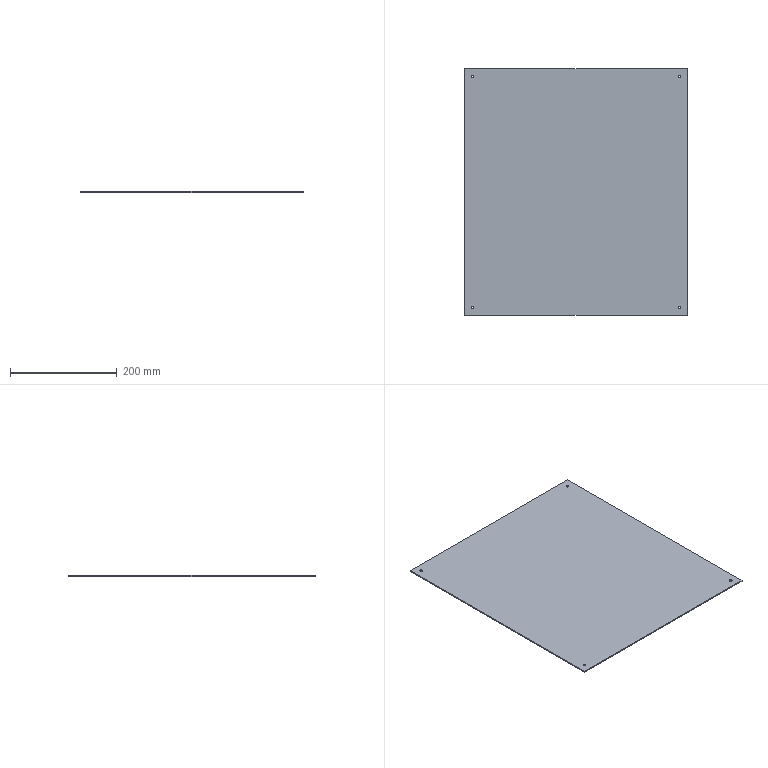Part | STEP file | PN_0004 (cover plate) | 1 solid | 14 faces | box 418 x 463 x 2 mm | volume 386911 mm3 | cylinder 8 | plane 6 | commonest cylinder face diameters 5 x8
STEP:
#1=CARTESIAN_POINT('',(0.,0.,0.));
#2=DIRECTION('',(0.,0.,1.));
#3=DIRECTION('',(1.,0.,0.));
#4=AXIS2_PLACEMENT_3D('',#1,#2,#3);
#5=CARTESIAN_POINT('',(-191.5,216.5,-2.));
#6=VERTEX_POINT('',#5);
#7=CARTESIAN_POINT('',(-191.5,216.5,0.));
#8=VERTEX_POINT('',#7);
#9=CARTESIAN_POINT('',(-191.5,216.5,0.));
#10=DIRECTION('',(0.,0.,1.));
#11=VECTOR('',#10,1.);
#12=LINE('',#9,#11);
#13=CARTESIAN_POINT('',(-194.,216.5,0.));
#14=DIRECTION('',(0.,0.,1.));
#15=DIRECTION('',(1.,0.,0.));
#16=AXIS2_PLACEMENT_3D('',#13,#14,#15);
#17=CYLINDRICAL_SURFACE('',#16,2.5);
#18=CARTESIAN_POINT('',(6.283,0.));
#19=DIRECTION('',(0.,1.));
#20=VECTOR('',#19,1.);
#21=LINE('',#18,#20);
#22=(GEOMETRIC_REPRESENTATION_CONTEXT(2)PARAMETRIC_REPRESENTATION_CONTEXT()REPRESENTATION_CONTEXT('',''));
#23=DEFINITIONAL_REPRESENTATION('',(#21),#22);
#24=PCURVE('',#17,#23);
#25=CARTESIAN_POINT('',(-194.,216.5,0.));
#26=DIRECTION('',(0.,0.,1.));
#27=DIRECTION('',(1.,0.,0.));
#28=AXIS2_PLACEMENT_3D('',#25,#26,#27);
#29=CYLINDRICAL_SURFACE('',#28,2.5);
#30=CARTESIAN_POINT('',(0.,0.));
#31=DIRECTION('',(0.,1.));
#32=VECTOR('',#31,1.);
#33=LINE('',#30,#32);
#34=(GEOMETRIC_REPRESENTATION_CONTEXT(2)PARAMETRIC_REPRESENTATION_CONTEXT()REPRESENTATION_CONTEXT('',''));
#35=DEFINITIONAL_REPRESENTATION('',(#33),#34);
#36=PCURVE('',#29,#35);
#37=SURFACE_CURVE('',#12,(#24,#36),.PCURVE_S1.);
#38=EDGE_CURVE('',#6,#8,#37,.T.);
#39=ORIENTED_EDGE('',*,*,#38,.T.);
#40=CARTESIAN_POINT('',(-196.5,216.5,0.));
#41=VERTEX_POINT('',#40);
#42=CARTESIAN_POINT('',(-194.,216.5,0.));
#43=DIRECTION('',(0.,0.,1.));
#44=DIRECTION('',(1.,0.,0.));
#45=AXIS2_PLACEMENT_3D('',#42,#43,#44);
#46=CIRCLE('',#45,2.5);
#47=CARTESIAN_POINT('',(0.,0.));
#48=DIRECTION('',(1.,0.));
#49=VECTOR('',#48,1.);
#50=LINE('',#47,#49);
#51=(GEOMETRIC_REPRESENTATION_CONTEXT(2)PARAMETRIC_REPRESENTATION_CONTEXT()REPRESENTATION_CONTEXT('',''));
#52=DEFINITIONAL_REPRESENTATION('',(#50),#51);
#53=PCURVE('',#17,#52);
#54=CARTESIAN_POINT('',(0.,0.,0.));
#55=DIRECTION('',(0.,0.,1.));
#56=DIRECTION('',(1.,0.,0.));
#57=AXIS2_PLACEMENT_3D('',#54,#55,#56);
#58=PLANE('',#57);
#59=CARTESIAN_POINT('',(-194.,216.5));
#60=DIRECTION('',(1.,0.));
#61=AXIS2_PLACEMENT_2D('',#59,#60);
#62=CIRCLE('',#61,2.5);
#63=(GEOMETRIC_REPRESENTATION_CONTEXT(2)PARAMETRIC_REPRESENTATION_CONTEXT()REPRESENTATION_CONTEXT('',''));
#64=DEFINITIONAL_REPRESENTATION('',(#62),#63);
#65=PCURVE('',#58,#64);
#66=SURFACE_CURVE('',#46,(#53,#65),.PCURVE_S1.);
#67=EDGE_CURVE('',#41,#8,#66,.T.);
#68=ORIENTED_EDGE('',*,*,#67,.F.);
#69=CARTESIAN_POINT('',(-196.5,216.5,-2.));
#70=VERTEX_POINT('',#69);
#71=CARTESIAN_POINT('',(-196.5,216.5,0.));
#72=DIRECTION('',(0.,0.,1.));
#73=VECTOR('',#72,1.);
#74=LINE('',#71,#73);
#75=CARTESIAN_POINT('',(3.142,0.));
#76=DIRECTION('',(0.,1.));
#77=VECTOR('',#76,1.);
#78=LINE('',#75,#77);
#79=(GEOMETRIC_REPRESENTATION_CONTEXT(2)PARAMETRIC_REPRESENTATION_CONTEXT()REPRESENTATION_CONTEXT('',''));
#80=DEFINITIONAL_REPRESENTATION('',(#78),#79);
#81=PCURVE('',#17,#80);
#82=CARTESIAN_POINT('',(3.142,0.));
#83=DIRECTION('',(0.,1.));
#84=VECTOR('',#83,1.);
#85=LINE('',#82,#84);
#86=(GEOMETRIC_REPRESENTATION_CONTEXT(2)PARAMETRIC_REPRESENTATION_CONTEXT()REPRESENTATION_CONTEXT('',''));
#87=DEFINITIONAL_REPRESENTATION('',(#85),#86);
#88=PCURVE('',#29,#87);
#89=SURFACE_CURVE('',#74,(#81,#88),.PCURVE_S1.);
#90=EDGE_CURVE('',#70,#41,#89,.T.);
#91=ORIENTED_EDGE('',*,*,#90,.F.);
#92=CARTESIAN_POINT('',(-194.,216.5,-2.));
#93=DIRECTION('',(0.,0.,1.));
#94=DIRECTION('',(1.,0.,0.));
#95=AXIS2_PLACEMENT_3D('',#92,#93,#94);
#96=CIRCLE('',#95,2.5);
#97=CARTESIAN_POINT('',(0.,-2.));
#98=DIRECTION('',(1.,0.));
#99=VECTOR('',#98,1.);
#100=LINE('',#97,#99);
#101=(GEOMETRIC_REPRESENTATION_CONTEXT(2)PARAMETRIC_REPRESENTATION_CONTEXT()REPRESENTATION_CONTEXT('',''));
#102=DEFINITIONAL_REPRESENTATION('',(#100),#101);
#103=PCURVE('',#17,#102);
#104=CARTESIAN_POINT('',(0.,0.,-2.));
#105=DIRECTION('',(0.,0.,1.));
#106=DIRECTION('',(1.,0.,0.));
#107=AXIS2_PLACEMENT_3D('',#104,#105,#106);
#108=PLANE('',#107);
#109=CARTESIAN_POINT('',(-194.,216.5));
#110=DIRECTION('',(1.,0.));
#111=AXIS2_PLACEMENT_2D('',#109,#110);
#112=CIRCLE('',#111,2.5);
#113=(GEOMETRIC_REPRESENTATION_CONTEXT(2)PARAMETRIC_REPRESENTATION_CONTEXT()REPRESENTATION_CONTEXT('',''));
#114=DEFINITIONAL_REPRESENTATION('',(#112),#113);
#115=PCURVE('',#108,#114);
#116=SURFACE_CURVE('',#96,(#103,#115),.PCURVE_S1.);
#117=EDGE_CURVE('',#70,#6,#116,.T.);
#118=ORIENTED_EDGE('',*,*,#117,.T.);
#119=EDGE_LOOP('',(#39,#68,#91,#118));
#120=FACE_BOUND('',#119,.F.);
#121=ADVANCED_FACE('',(#120),#17,.F.);
#122=CARTESIAN_POINT('',(-191.5,-216.5,-2.));
#123=VERTEX_POINT('',#122);
#124=CARTESIAN_POINT('',(-191.5,-216.5,0.));
#125=VERTEX_POINT('',#124);
#126=CARTESIAN_POINT('',(-191.5,-216.5,0.));
#127=DIRECTION('',(0.,0.,1.));
#128=VECTOR('',#127,1.);
#129=LINE('',#126,#128);
#130=CARTESIAN_POINT('',(-194.,-216.5,0.));
#131=DIRECTION('',(0.,0.,1.));
#132=DIRECTION('',(1.,0.,0.));
#133=AXIS2_PLACEMENT_3D('',#130,#131,#132);
#134=CYLINDRICAL_SURFACE('',#133,2.5);
#135=CARTESIAN_POINT('',(6.283,0.));
#136=DIRECTION('',(0.,1.));
#137=VECTOR('',#136,1.);
#138=LINE('',#135,#137);
#139=(GEOMETRIC_REPRESENTATION_CONTEXT(2)PARAMETRIC_REPRESENTATION_CONTEXT()REPRESENTATION_CONTEXT('',''));
#140=DEFINITIONAL_REPRESENTATION('',(#138),#139);
#141=PCURVE('',#134,#140);
#142=CARTESIAN_POINT('',(-194.,-216.5,0.));
#143=DIRECTION('',(0.,0.,1.));
#144=DIRECTION('',(1.,0.,0.));
#145=AXIS2_PLACEMENT_3D('',#142,#143,#144);
#146=CYLINDRICAL_SURFACE('',#145,2.5);
#147=CARTESIAN_POINT('',(0.,0.));
#148=DIRECTION('',(0.,1.));
#149=VECTOR('',#148,1.);
#150=LINE('',#147,#149);
#151=(GEOMETRIC_REPRESENTATION_CONTEXT(2)PARAMETRIC_REPRESENTATION_CONTEXT()REPRESENTATION_CONTEXT('',''));
#152=DEFINITIONAL_REPRESENTATION('',(#150),#151);
#153=PCURVE('',#146,#152);
#154=SURFACE_CURVE('',#129,(#141,#153),.PCURVE_S1.);
#155=EDGE_CURVE('',#123,#125,#154,.T.);
#156=ORIENTED_EDGE('',*,*,#155,.T.);
#157=CARTESIAN_POINT('',(-196.5,-216.5,0.));
#158=VERTEX_POINT('',#157);
#159=CARTESIAN_POINT('',(-194.,-216.5,0.));
#160=DIRECTION('',(0.,0.,1.));
#161=DIRECTION('',(1.,0.,0.));
#162=AXIS2_PLACEMENT_3D('',#159,#160,#161);
#163=CIRCLE('',#162,2.5);
#164=CARTESIAN_POINT('',(0.,0.));
#165=DIRECTION('',(1.,0.));
#166=VECTOR('',#165,1.);
#167=LINE('',#164,#166);
#168=(GEOMETRIC_REPRESENTATION_CONTEXT(2)PARAMETRIC_REPRESENTATION_CONTEXT()REPRESENTATION_CONTEXT('',''));
#169=DEFINITIONAL_REPRESENTATION('',(#167),#168);
#170=PCURVE('',#134,#169);
#171=CARTESIAN_POINT('',(-194.,-216.5));
#172=DIRECTION('',(1.,0.));
#173=AXIS2_PLACEMENT_2D('',#171,#172);
#174=CIRCLE('',#173,2.5);
#175=(GEOMETRIC_REPRESENTATION_CONTEXT(2)PARAMETRIC_REPRESENTATION_CONTEXT()REPRESENTATION_CONTEXT('',''));
#176=DEFINITIONAL_REPRESENTATION('',(#174),#175);
#177=PCURVE('',#58,#176);
#178=SURFACE_CURVE('',#163,(#170,#177),.PCURVE_S1.);
#179=EDGE_CURVE('',#158,#125,#178,.T.);
#180=ORIENTED_EDGE('',*,*,#179,.F.);
#181=CARTESIAN_POINT('',(-196.5,-216.5,-2.));
#182=VERTEX_POINT('',#181);
#183=CARTESIAN_POINT('',(-196.5,-216.5,0.));
#184=DIRECTION('',(0.,0.,1.));
#185=VECTOR('',#184,1.);
#186=LINE('',#183,#185);
#187=CARTESIAN_POINT('',(3.142,0.));
#188=DIRECTION('',(0.,1.));
#189=VECTOR('',#188,1.);
#190=LINE('',#187,#189);
#191=(GEOMETRIC_REPRESENTATION_CONTEXT(2)PARAMETRIC_REPRESENTATION_CONTEXT()REPRESENTATION_CONTEXT('',''));
#192=DEFINITIONAL_REPRESENTATION('',(#190),#191);
#193=PCURVE('',#134,#192);
#194=CARTESIAN_POINT('',(3.142,0.));
#195=DIRECTION('',(0.,1.));
#196=VECTOR('',#195,1.);
#197=LINE('',#194,#196);
#198=(GEOMETRIC_REPRESENTATION_CONTEXT(2)PARAMETRIC_REPRESENTATION_CONTEXT()REPRESENTATION_CONTEXT('',''));
#199=DEFINITIONAL_REPRESENTATION('',(#197),#198);
#200=PCURVE('',#146,#199);
#201=SURFACE_CURVE('',#186,(#193,#200),.PCURVE_S1.);
#202=EDGE_CURVE('',#182,#158,#201,.T.);
#203=ORIENTED_EDGE('',*,*,#202,.F.);
#204=CARTESIAN_POINT('',(-194.,-216.5,-2.));
#205=DIRECTION('',(0.,0.,1.));
#206=DIRECTION('',(1.,0.,0.));
#207=AXIS2_PLACEMENT_3D('',#204,#205,#206);
#208=CIRCLE('',#207,2.5);
#209=CARTESIAN_POINT('',(0.,-2.));
#210=DIRECTION('',(1.,0.));
#211=VECTOR('',#210,1.);
#212=LINE('',#209,#211);
#213=(GEOMETRIC_REPRESENTATION_CONTEXT(2)PARAMETRIC_REPRESENTATION_CONTEXT()REPRESENTATION_CONTEXT('',''));
#214=DEFINITIONAL_REPRESENTATION('',(#212),#213);
#215=PCURVE('',#134,#214);
#216=CARTESIAN_POINT('',(-194.,-216.5));
#217=DIRECTION('',(1.,0.));
#218=AXIS2_PLACEMENT_2D('',#216,#217);
#219=CIRCLE('',#218,2.5);
#220=(GEOMETRIC_REPRESENTATION_CONTEXT(2)PARAMETRIC_REPRESENTATION_CONTEXT()REPRESENTATION_CONTEXT('',''));
#221=DEFINITIONAL_REPRESENTATION('',(#219),#220);
#222=PCURVE('',#108,#221);
#223=SURFACE_CURVE('',#208,(#215,#222),.PCURVE_S1.);
#224=EDGE_CURVE('',#182,#123,#223,.T.);
#225=ORIENTED_EDGE('',*,*,#224,.T.);
#226=EDGE_LOOP('',(#156,#180,#203,#225));
#227=FACE_BOUND('',#226,.F.);
#228=ADVANCED_FACE('',(#227),#134,.F.);
#229=CARTESIAN_POINT('',(196.5,-216.5,-2.));
#230=VERTEX_POINT('',#229);
#231=CARTESIAN_POINT('',(196.5,-216.5,0.));
#232=VERTEX_POINT('',#231);
#233=CARTESIAN_POINT('',(196.5,-216.5,0.));
#234=DIRECTION('',(0.,0.,1.));
#235=VECTOR('',#234,1.);
#236=LINE('',#233,#235);
#237=CARTESIAN_POINT('',(194.,-216.5,0.));
#238=DIRECTION('',(0.,0.,1.));
#239=DIRECTION('',(1.,0.,0.));
#240=AXIS2_PLACEMENT_3D('',#237,#238,#239);
#241=CYLINDRICAL_SURFACE('',#240,2.5);
#242=CARTESIAN_POINT('',(6.283,0.));
#243=DIRECTION('',(0.,1.));
#244=VECTOR('',#243,1.);
#245=LINE('',#242,#244);
#246=(GEOMETRIC_REPRESENTATION_CONTEXT(2)PARAMETRIC_REPRESENTATION_CONTEXT()REPRESENTATION_CONTEXT('',''));
#247=DEFINITIONAL_REPRESENTATION('',(#245),#246);
#248=PCURVE('',#241,#247);
#249=CARTESIAN_POINT('',(194.,-216.5,0.));
#250=DIRECTION('',(0.,0.,1.));
#251=DIRECTION('',(1.,0.,0.));
#252=AXIS2_PLACEMENT_3D('',#249,#250,#251);
#253=CYLINDRICAL_SURFACE('',#252,2.5);
#254=CARTESIAN_POINT('',(0.,0.));
#255=DIRECTION('',(0.,1.));
#256=VECTOR('',#255,1.);
#257=LINE('',#254,#256);
#258=(GEOMETRIC_REPRESENTATION_CONTEXT(2)PARAMETRIC_REPRESENTATION_CONTEXT()REPRESENTATION_CONTEXT('',''));
#259=DEFINITIONAL_REPRESENTATION('',(#257),#258);
#260=PCURVE('',#253,#259);
#261=SURFACE_CURVE('',#236,(#248,#260),.PCURVE_S1.);
#262=EDGE_CURVE('',#230,#232,#261,.T.);
#263=ORIENTED_EDGE('',*,*,#262,.T.);
#264=CARTESIAN_POINT('',(191.5,-216.5,0.));
#265=VERTEX_POINT('',#264);
#266=CARTESIAN_POINT('',(194.,-216.5,0.));
#267=DIRECTION('',(0.,0.,1.));
#268=DIRECTION('',(1.,0.,0.));
#269=AXIS2_PLACEMENT_3D('',#266,#267,#268);
#270=CIRCLE('',#269,2.5);
#271=CARTESIAN_POINT('',(0.,0.));
#272=DIRECTION('',(1.,0.));
#273=VECTOR('',#272,1.);
#274=LINE('',#271,#273);
#275=(GEOMETRIC_REPRESENTATION_CONTEXT(2)PARAMETRIC_REPRESENTATION_CONTEXT()REPRESENTATION_CONTEXT('',''));
#276=DEFINITIONAL_REPRESENTATION('',(#274),#275);
#277=PCURVE('',#241,#276);
#278=CARTESIAN_POINT('',(194.,-216.5));
#279=DIRECTION('',(1.,0.));
#280=AXIS2_PLACEMENT_2D('',#278,#279);
#281=CIRCLE('',#280,2.5);
#282=(GEOMETRIC_REPRESENTATION_CONTEXT(2)PARAMETRIC_REPRESENTATION_CONTEXT()REPRESENTATION_CONTEXT('',''));
#283=DEFINITIONAL_REPRESENTATION('',(#281),#282);
#284=PCURVE('',#58,#283);
#285=SURFACE_CURVE('',#270,(#277,#284),.PCURVE_S1.);
#286=EDGE_CURVE('',#265,#232,#285,.T.);
#287=ORIENTED_EDGE('',*,*,#286,.F.);
#288=CARTESIAN_POINT('',(191.5,-216.5,-2.));
#289=VERTEX_POINT('',#288);
#290=CARTESIAN_POINT('',(191.5,-216.5,0.));
#291=DIRECTION('',(0.,0.,1.));
#292=VECTOR('',#291,1.);
#293=LINE('',#290,#292);
#294=CARTESIAN_POINT('',(3.142,0.));
#295=DIRECTION('',(0.,1.));
#296=VECTOR('',#295,1.);
#297=LINE('',#294,#296);
#298=(GEOMETRIC_REPRESENTATION_CONTEXT(2)PARAMETRIC_REPRESENTATION_CONTEXT()REPRESENTATION_CONTEXT('',''));
#299=DEFINITIONAL_REPRESENTATION('',(#297),#298);
#300=PCURVE('',#241,#299);
#301=CARTESIAN_POINT('',(3.142,0.));
#302=DIRECTION('',(0.,1.));
#303=VECTOR('',#302,1.);
#304=LINE('',#301,#303);
#305=(GEOMETRIC_REPRESENTATION_CONTEXT(2)PARAMETRIC_REPRESENTATION_CONTEXT()REPRESENTATION_CONTEXT('',''));
#306=DEFINITIONAL_REPRESENTATION('',(#304),#305);
#307=PCURVE('',#253,#306);
#308=SURFACE_CURVE('',#293,(#300,#307),.PCURVE_S1.);
#309=EDGE_CURVE('',#289,#265,#308,.T.);
#310=ORIENTED_EDGE('',*,*,#309,.F.);
#311=CARTESIAN_POINT('',(194.,-216.5,-2.));
#312=DIRECTION('',(0.,0.,1.));
#313=DIRECTION('',(1.,0.,0.));
#314=AXIS2_PLACEMENT_3D('',#311,#312,#313);
#315=CIRCLE('',#314,2.5);
#316=CARTESIAN_POINT('',(0.,-2.));
#317=DIRECTION('',(1.,0.));
#318=VECTOR('',#317,1.);
#319=LINE('',#316,#318);
#320=(GEOMETRIC_REPRESENTATION_CONTEXT(2)PARAMETRIC_REPRESENTATION_CONTEXT()REPRESENTATION_CONTEXT('',''));
#321=DEFINITIONAL_REPRESENTATION('',(#319),#320);
#322=PCURVE('',#241,#321);
#323=CARTESIAN_POINT('',(194.,-216.5));
#324=DIRECTION('',(1.,0.));
#325=AXIS2_PLACEMENT_2D('',#323,#324);
#326=CIRCLE('',#325,2.5);
#327=(GEOMETRIC_REPRESENTATION_CONTEXT(2)PARAMETRIC_REPRESENTATION_CONTEXT()REPRESENTATION_CONTEXT('',''));
#328=DEFINITIONAL_REPRESENTATION('',(#326),#327);
#329=PCURVE('',#108,#328);
#330=SURFACE_CURVE('',#315,(#322,#329),.PCURVE_S1.);
#331=EDGE_CURVE('',#289,#230,#330,.T.);
#332=ORIENTED_EDGE('',*,*,#331,.T.);
#333=EDGE_LOOP('',(#263,#287,#310,#332));
#334=FACE_BOUND('',#333,.F.);
#335=ADVANCED_FACE('',(#334),#241,.F.);
#336=CARTESIAN_POINT('',(196.5,216.5,-2.));
#337=VERTEX_POINT('',#336);
#338=CARTESIAN_POINT('',(196.5,216.5,0.));
#339=VERTEX_POINT('',#338);
#340=CARTESIAN_POINT('',(196.5,216.5,0.));
#341=DIRECTION('',(0.,0.,1.));
#342=VECTOR('',#341,1.);
#343=LINE('',#340,#342);
#344=CARTESIAN_POINT('',(194.,216.5,0.));
#345=DIRECTION('',(0.,0.,1.));
#346=DIRECTION('',(1.,0.,0.));
#347=AXIS2_PLACEMENT_3D('',#344,#345,#346);
#348=CYLINDRICAL_SURFACE('',#347,2.5);
#349=CARTESIAN_POINT('',(6.283,0.));
#350=DIRECTION('',(0.,1.));
#351=VECTOR('',#350,1.);
#352=LINE('',#349,#351);
#353=(GEOMETRIC_REPRESENTATION_CONTEXT(2)PARAMETRIC_REPRESENTATION_CONTEXT()REPRESENTATION_CONTEXT('',''));
#354=DEFINITIONAL_REPRESENTATION('',(#352),#353);
#355=PCURVE('',#348,#354);
#356=CARTESIAN_POINT('',(194.,216.5,0.));
#357=DIRECTION('',(0.,0.,1.));
#358=DIRECTION('',(1.,0.,0.));
#359=AXIS2_PLACEMENT_3D('',#356,#357,#358);
#360=CYLINDRICAL_SURFACE('',#359,2.5);
#361=CARTESIAN_POINT('',(0.,0.));
#362=DIRECTION('',(0.,1.));
#363=VECTOR('',#362,1.);
#364=LINE('',#361,#363);
#365=(GEOMETRIC_REPRESENTATION_CONTEXT(2)PARAMETRIC_REPRESENTATION_CONTEXT()REPRESENTATION_CONTEXT('',''));
#366=DEFINITIONAL_REPRESENTATION('',(#364),#365);
#367=PCURVE('',#360,#366);
#368=SURFACE_CURVE('',#343,(#355,#367),.PCURVE_S1.);
#369=EDGE_CURVE('',#337,#339,#368,.T.);
#370=ORIENTED_EDGE('',*,*,#369,.T.);
#371=CARTESIAN_POINT('',(191.5,216.5,0.));
#372=VERTEX_POINT('',#371);
#373=CARTESIAN_POINT('',(194.,216.5,0.));
#374=DIRECTION('',(0.,0.,1.));
#375=DIRECTION('',(1.,0.,0.));
#376=AXIS2_PLACEMENT_3D('',#373,#374,#375);
#377=CIRCLE('',#376,2.5);
#378=CARTESIAN_POINT('',(0.,0.));
#379=DIRECTION('',(1.,0.));
#380=VECTOR('',#379,1.);
#381=LINE('',#378,#380);
#382=(GEOMETRIC_REPRESENTATION_CONTEXT(2)PARAMETRIC_REPRESENTATION_CONTEXT()REPRESENTATION_CONTEXT('',''));
#383=DEFINITIONAL_REPRESENTATION('',(#381),#382);
#384=PCURVE('',#348,#383);
#385=CARTESIAN_POINT('',(194.,216.5));
#386=DIRECTION('',(1.,0.));
#387=AXIS2_PLACEMENT_2D('',#385,#386);
#388=CIRCLE('',#387,2.5);
#389=(GEOMETRIC_REPRESENTATION_CONTEXT(2)PARAMETRIC_REPRESENTATION_CONTEXT()REPRESENTATION_CONTEXT('',''));
#390=DEFINITIONAL_REPRESENTATION('',(#388),#389);
#391=PCURVE('',#58,#390);
#392=SURFACE_CURVE('',#377,(#384,#391),.PCURVE_S1.);
#393=EDGE_CURVE('',#372,#339,#392,.T.);
#394=ORIENTED_EDGE('',*,*,#393,.F.);
#395=CARTESIAN_POINT('',(191.5,216.5,-2.));
#396=VERTEX_POINT('',#395);
#397=CARTESIAN_POINT('',(191.5,216.5,0.));
#398=DIRECTION('',(0.,0.,1.));
#399=VECTOR('',#398,1.);
#400=LINE('',#397,#399);
#401=CARTESIAN_POINT('',(3.142,0.));
#402=DIRECTION('',(0.,1.));
#403=VECTOR('',#402,1.);
#404=LINE('',#401,#403);
#405=(GEOMETRIC_REPRESENTATION_CONTEXT(2)PARAMETRIC_REPRESENTATION_CONTEXT()REPRESENTATION_CONTEXT('',''));
#406=DEFINITIONAL_REPRESENTATION('',(#404),#405);
#407=PCURVE('',#348,#406);
#408=CARTESIAN_POINT('',(3.142,0.));
#409=DIRECTION('',(0.,1.));
#410=VECTOR('',#409,1.);
#411=LINE('',#408,#410);
#412=(GEOMETRIC_REPRESENTATION_CONTEXT(2)PARAMETRIC_REPRESENTATION_CONTEXT()REPRESENTATION_CONTEXT('',''));
#413=DEFINITIONAL_REPRESENTATION('',(#411),#412);
#414=PCURVE('',#360,#413);
#415=SURFACE_CURVE('',#400,(#407,#414),.PCURVE_S1.);
#416=EDGE_CURVE('',#396,#372,#415,.T.);
#417=ORIENTED_EDGE('',*,*,#416,.F.);
#418=CARTESIAN_POINT('',(194.,216.5,-2.));
#419=DIRECTION('',(0.,0.,1.));
#420=DIRECTION('',(1.,0.,0.));
#421=AXIS2_PLACEMENT_3D('',#418,#419,#420);
#422=CIRCLE('',#421,2.5);
#423=CARTESIAN_POINT('',(0.,-2.));
#424=DIRECTION('',(1.,0.));
#425=VECTOR('',#424,1.);
#426=LINE('',#423,#425);
#427=(GEOMETRIC_REPRESENTATION_CONTEXT(2)PARAMETRIC_REPRESENTATION_CONTEXT()REPRESENTATION_CONTEXT('',''));
#428=DEFINITIONAL_REPRESENTATION('',(#426),#427);
#429=PCURVE('',#348,#428);
#430=CARTESIAN_POINT('',(194.,216.5));
#431=DIRECTION('',(1.,0.));
#432=AXIS2_PLACEMENT_2D('',#430,#431);
#433=CIRCLE('',#432,2.5);
#434=(GEOMETRIC_REPRESENTATION_CONTEXT(2)PARAMETRIC_REPRESENTATION_CONTEXT()REPRESENTATION_CONTEXT('',''));
#435=DEFINITIONAL_REPRESENTATION('',(#433),#434);
#436=PCURVE('',#108,#435);
#437=SURFACE_CURVE('',#422,(#429,#436),.PCURVE_S1.);
#438=EDGE_CURVE('',#396,#337,#437,.T.);
#439=ORIENTED_EDGE('',*,*,#438,.T.);
#440=EDGE_LOOP('',(#370,#394,#417,#439));
#441=FACE_BOUND('',#440,.F.);
#442=ADVANCED_FACE('',(#441),#348,.F.);
#443=CARTESIAN_POINT('',(-209.,231.5,0.));
#444=VERTEX_POINT('',#443);
#445=CARTESIAN_POINT('',(-209.,-231.5,0.));
#446=VERTEX_POINT('',#445);
#447=CARTESIAN_POINT('',(-209.,-231.5,0.));
#448=DIRECTION('',(0.,-1.,0.));
#449=VECTOR('',#448,1.);
#450=LINE('',#447,#449);
#451=CARTESIAN_POINT('',(-209.,-231.5,-2.));
#452=DIRECTION('',(-1.,0.,0.));
#453=DIRECTION('',(0.,0.,1.));
#454=AXIS2_PLACEMENT_3D('',#451,#452,#453);
#455=PLANE('',#454);
#456=CARTESIAN_POINT('',(2.,0.));
#457=DIRECTION('',(0.,-1.));
#458=VECTOR('',#457,1.);
#459=LINE('',#456,#458);
#460=(GEOMETRIC_REPRESENTATION_CONTEXT(2)PARAMETRIC_REPRESENTATION_CONTEXT()REPRESENTATION_CONTEXT('',''));
#461=DEFINITIONAL_REPRESENTATION('',(#459),#460);
#462=PCURVE('',#455,#461);
#463=CARTESIAN_POINT('',(-209.,-231.5));
#464=DIRECTION('',(0.,-1.));
#465=VECTOR('',#464,1.);
#466=LINE('',#463,#465);
#467=(GEOMETRIC_REPRESENTATION_CONTEXT(2)PARAMETRIC_REPRESENTATION_CONTEXT()REPRESENTATION_CONTEXT('',''));
#468=DEFINITIONAL_REPRESENTATION('',(#466),#467);
#469=PCURVE('',#58,#468);
#470=SURFACE_CURVE('',#450,(#462,#469),.PCURVE_S1.);
#471=EDGE_CURVE('',#444,#446,#470,.T.);
#472=ORIENTED_EDGE('',*,*,#471,.F.);
#473=CARTESIAN_POINT('',(-209.,231.5,-2.));
#474=VERTEX_POINT('',#473);
#475=CARTESIAN_POINT('',(-209.,231.5,-2.));
#476=DIRECTION('',(0.,0.,1.));
#477=VECTOR('',#476,1.);
#478=LINE('',#475,#477);
#479=CARTESIAN_POINT('',(0.,463.));
#480=DIRECTION('',(1.,0.));
#481=VECTOR('',#480,1.);
#482=LINE('',#479,#481);
#483=(GEOMETRIC_REPRESENTATION_CONTEXT(2)PARAMETRIC_REPRESENTATION_CONTEXT()REPRESENTATION_CONTEXT('',''));
#484=DEFINITIONAL_REPRESENTATION('',(#482),#483);
#485=PCURVE('',#455,#484);
#486=CARTESIAN_POINT('',(209.,231.5,-2.));
#487=DIRECTION('',(0.,1.,0.));
#488=DIRECTION('',(-1.,0.,0.));
#489=AXIS2_PLACEMENT_3D('',#486,#487,#488);
#490=PLANE('',#489);
#491=CARTESIAN_POINT('',(418.,0.));
#492=DIRECTION('',(0.,1.));
#493=VECTOR('',#492,1.);
#494=LINE('',#491,#493);
#495=(GEOMETRIC_REPRESENTATION_CONTEXT(2)PARAMETRIC_REPRESENTATION_CONTEXT()REPRESENTATION_CONTEXT('',''));
#496=DEFINITIONAL_REPRESENTATION('',(#494),#495);
#497=PCURVE('',#490,#496);
#498=SURFACE_CURVE('',#478,(#485,#497),.PCURVE_S1.);
#499=EDGE_CURVE('',#474,#444,#498,.T.);
#500=ORIENTED_EDGE('',*,*,#499,.F.);
#501=CARTESIAN_POINT('',(-209.,-231.5,-2.));
#502=VERTEX_POINT('',#501);
#503=CARTESIAN_POINT('',(-209.,-231.5,-2.));
#504=DIRECTION('',(0.,-1.,0.));
#505=VECTOR('',#504,1.);
#506=LINE('',#503,#505);
#507=CARTESIAN_POINT('',(0.,0.));
#508=DIRECTION('',(0.,-1.));
#509=VECTOR('',#508,1.);
#510=LINE('',#507,#509);
#511=(GEOMETRIC_REPRESENTATION_CONTEXT(2)PARAMETRIC_REPRESENTATION_CONTEXT()REPRESENTATION_CONTEXT('',''));
#512=DEFINITIONAL_REPRESENTATION('',(#510),#511);
#513=PCURVE('',#455,#512);
#514=CARTESIAN_POINT('',(-209.,-231.5));
#515=DIRECTION('',(0.,-1.));
#516=VECTOR('',#515,1.);
#517=LINE('',#514,#516);
#518=(GEOMETRIC_REPRESENTATION_CONTEXT(2)PARAMETRIC_REPRESENTATION_CONTEXT()REPRESENTATION_CONTEXT('',''));
#519=DEFINITIONAL_REPRESENTATION('',(#517),#518);
#520=PCURVE('',#108,#519);
#521=SURFACE_CURVE('',#506,(#513,#520),.PCURVE_S1.);
#522=EDGE_CURVE('',#474,#502,#521,.T.);
#523=ORIENTED_EDGE('',*,*,#522,.T.);
#524=CARTESIAN_POINT('',(-209.,-231.5,-2.));
#525=DIRECTION('',(0.,0.,1.));
#526=VECTOR('',#525,1.);
#527=LINE('',#524,#526);
#528=CARTESIAN_POINT('',(0.,0.));
#529=DIRECTION('',(1.,0.));
#530=VECTOR('',#529,1.);
#531=LINE('',#528,#530);
#532=(GEOMETRIC_REPRESENTATION_CONTEXT(2)PARAMETRIC_REPRESENTATION_CONTEXT()REPRESENTATION_CONTEXT('',''));
#533=DEFINITIONAL_REPRESENTATION('',(#531),#532);
#534=PCURVE('',#455,#533);
#535=CARTESIAN_POINT('',(209.,-231.5,-2.));
#536=DIRECTION('',(0.,-1.,0.));
#537=DIRECTION('',(1.,0.,0.));
#538=AXIS2_PLACEMENT_3D('',#535,#536,#537);
#539=PLANE('',#538);
#540=CARTESIAN_POINT('',(-418.,0.));
#541=DIRECTION('',(0.,1.));
#542=VECTOR('',#541,1.);
#543=LINE('',#540,#542);
#544=(GEOMETRIC_REPRESENTATION_CONTEXT(2)PARAMETRIC_REPRESENTATION_CONTEXT()REPRESENTATION_CONTEXT('',''));
#545=DEFINITIONAL_REPRESENTATION('',(#543),#544);
#546=PCURVE('',#539,#545);
#547=SURFACE_CURVE('',#527,(#534,#546),.PCURVE_S1.);
#548=EDGE_CURVE('',#502,#446,#547,.T.);
#549=ORIENTED_EDGE('',*,*,#548,.T.);
#550=EDGE_LOOP('',(#472,#500,#523,#549));
#551=FACE_BOUND('',#550,.T.);
#552=ADVANCED_FACE('',(#551),#455,.T.);
#553=CARTESIAN_POINT('',(209.,231.5,0.));
#554=VERTEX_POINT('',#553);
#555=CARTESIAN_POINT('',(209.,231.5,0.));
#556=DIRECTION('',(-1.,0.,0.));
#557=VECTOR('',#556,1.);
#558=LINE('',#555,#557);
#559=CARTESIAN_POINT('',(0.,2.));
#560=DIRECTION('',(1.,0.));
#561=VECTOR('',#560,1.);
#562=LINE('',#559,#561);
#563=(GEOMETRIC_REPRESENTATION_CONTEXT(2)PARAMETRIC_REPRESENTATION_CONTEXT()REPRESENTATION_CONTEXT('',''));
#564=DEFINITIONAL_REPRESENTATION('',(#562),#563);
#565=PCURVE('',#490,#564);
#566=CARTESIAN_POINT('',(209.,231.5));
#567=DIRECTION('',(-1.,0.));
#568=VECTOR('',#567,1.);
#569=LINE('',#566,#568);
#570=(GEOMETRIC_REPRESENTATION_CONTEXT(2)PARAMETRIC_REPRESENTATION_CONTEXT()REPRESENTATION_CONTEXT('',''));
#571=DEFINITIONAL_REPRESENTATION('',(#569),#570);
#572=PCURVE('',#58,#571);
#573=SURFACE_CURVE('',#558,(#565,#572),.PCURVE_S1.);
#574=EDGE_CURVE('',#554,#444,#573,.T.);
#575=ORIENTED_EDGE('',*,*,#574,.F.);
#576=CARTESIAN_POINT('',(209.,231.5,-2.));
#577=VERTEX_POINT('',#576);
#578=CARTESIAN_POINT('',(209.,231.5,-2.));
#579=DIRECTION('',(0.,0.,1.));
#580=VECTOR('',#579,1.);
#581=LINE('',#578,#580);
#582=CARTESIAN_POINT('',(0.,0.));
#583=DIRECTION('',(0.,1.));
#584=VECTOR('',#583,1.);
#585=LINE('',#582,#584);
#586=(GEOMETRIC_REPRESENTATION_CONTEXT(2)PARAMETRIC_REPRESENTATION_CONTEXT()REPRESENTATION_CONTEXT('',''));
#587=DEFINITIONAL_REPRESENTATION('',(#585),#586);
#588=PCURVE('',#490,#587);
#589=CARTESIAN_POINT('',(209.,-231.5,-2.));
#590=DIRECTION('',(1.,0.,0.));
#591=DIRECTION('',(0.,0.,-1.));
#592=AXIS2_PLACEMENT_3D('',#589,#590,#591);
#593=PLANE('',#592);
#594=CARTESIAN_POINT('',(0.,463.));
#595=DIRECTION('',(-1.,0.));
#596=VECTOR('',#595,1.);
#597=LINE('',#594,#596);
#598=(GEOMETRIC_REPRESENTATION_CONTEXT(2)PARAMETRIC_REPRESENTATION_CONTEXT()REPRESENTATION_CONTEXT('',''));
#599=DEFINITIONAL_REPRESENTATION('',(#597),#598);
#600=PCURVE('',#593,#599);
#601=SURFACE_CURVE('',#581,(#588,#600),.PCURVE_S1.);
#602=EDGE_CURVE('',#577,#554,#601,.T.);
#603=ORIENTED_EDGE('',*,*,#602,.F.);
#604=CARTESIAN_POINT('',(209.,231.5,-2.));
#605=DIRECTION('',(-1.,0.,0.));
#606=VECTOR('',#605,1.);
#607=LINE('',#604,#606);
#608=CARTESIAN_POINT('',(0.,0.));
#609=DIRECTION('',(1.,0.));
#610=VECTOR('',#609,1.);
#611=LINE('',#608,#610);
#612=(GEOMETRIC_REPRESENTATION_CONTEXT(2)PARAMETRIC_REPRESENTATION_CONTEXT()REPRESENTATION_CONTEXT('',''));
#613=DEFINITIONAL_REPRESENTATION('',(#611),#612);
#614=PCURVE('',#490,#613);
#615=CARTESIAN_POINT('',(209.,231.5));
#616=DIRECTION('',(-1.,0.));
#617=VECTOR('',#616,1.);
#618=LINE('',#615,#617);
#619=(GEOMETRIC_REPRESENTATION_CONTEXT(2)PARAMETRIC_REPRESENTATION_CONTEXT()REPRESENTATION_CONTEXT('',''));
#620=DEFINITIONAL_REPRESENTATION('',(#618),#619);
#621=PCURVE('',#108,#620);
#622=SURFACE_CURVE('',#607,(#614,#621),.PCURVE_S1.);
#623=EDGE_CURVE('',#577,#474,#622,.T.);
#624=ORIENTED_EDGE('',*,*,#623,.T.);
#625=ORIENTED_EDGE('',*,*,#499,.T.);
#626=EDGE_LOOP('',(#575,#603,#624,#625));
#627=FACE_BOUND('',#626,.T.);
#628=ADVANCED_FACE('',(#627),#490,.T.);
#629=CARTESIAN_POINT('',(209.,-231.5,0.));
#630=VERTEX_POINT('',#629);
#631=CARTESIAN_POINT('',(209.,-231.5,0.));
#632=DIRECTION('',(0.,1.,0.));
#633=VECTOR('',#632,1.);
#634=LINE('',#631,#633);
#635=CARTESIAN_POINT('',(-2.,0.));
#636=DIRECTION('',(0.,1.));
#637=VECTOR('',#636,1.);
#638=LINE('',#635,#637);
#639=(GEOMETRIC_REPRESENTATION_CONTEXT(2)PARAMETRIC_REPRESENTATION_CONTEXT()REPRESENTATION_CONTEXT('',''));
#640=DEFINITIONAL_REPRESENTATION('',(#638),#639);
#641=PCURVE('',#593,#640);
#642=CARTESIAN_POINT('',(209.,-231.5));
#643=DIRECTION('',(0.,1.));
#644=VECTOR('',#643,1.);
#645=LINE('',#642,#644);
#646=(GEOMETRIC_REPRESENTATION_CONTEXT(2)PARAMETRIC_REPRESENTATION_CONTEXT()REPRESENTATION_CONTEXT('',''));
#647=DEFINITIONAL_REPRESENTATION('',(#645),#646);
#648=PCURVE('',#58,#647);
#649=SURFACE_CURVE('',#634,(#641,#648),.PCURVE_S1.);
#650=EDGE_CURVE('',#630,#554,#649,.T.);
#651=ORIENTED_EDGE('',*,*,#650,.F.);
#652=CARTESIAN_POINT('',(209.,-231.5,-2.));
#653=VERTEX_POINT('',#652);
#654=CARTESIAN_POINT('',(209.,-231.5,-2.));
#655=DIRECTION('',(0.,0.,1.));
#656=VECTOR('',#655,1.);
#657=LINE('',#654,#656);
#658=CARTESIAN_POINT('',(0.,0.));
#659=DIRECTION('',(-1.,0.));
#660=VECTOR('',#659,1.);
#661=LINE('',#658,#660);
#662=(GEOMETRIC_REPRESENTATION_CONTEXT(2)PARAMETRIC_REPRESENTATION_CONTEXT()REPRESENTATION_CONTEXT('',''));
#663=DEFINITIONAL_REPRESENTATION('',(#661),#662);
#664=PCURVE('',#593,#663);
#665=CARTESIAN_POINT('',(0.,0.));
#666=DIRECTION('',(0.,1.));
#667=VECTOR('',#666,1.);
#668=LINE('',#665,#667);
#669=(GEOMETRIC_REPRESENTATION_CONTEXT(2)PARAMETRIC_REPRESENTATION_CONTEXT()REPRESENTATION_CONTEXT('',''));
#670=DEFINITIONAL_REPRESENTATION('',(#668),#669);
#671=PCURVE('',#539,#670);
#672=SURFACE_CURVE('',#657,(#664,#671),.PCURVE_S1.);
#673=EDGE_CURVE('',#653,#630,#672,.T.);
#674=ORIENTED_EDGE('',*,*,#673,.F.);
#675=CARTESIAN_POINT('',(209.,-231.5,-2.));
#676=DIRECTION('',(0.,1.,0.));
#677=VECTOR('',#676,1.);
#678=LINE('',#675,#677);
#679=CARTESIAN_POINT('',(0.,0.));
#680=DIRECTION('',(0.,1.));
#681=VECTOR('',#680,1.);
#682=LINE('',#679,#681);
#683=(GEOMETRIC_REPRESENTATION_CONTEXT(2)PARAMETRIC_REPRESENTATION_CONTEXT()REPRESENTATION_CONTEXT('',''));
#684=DEFINITIONAL_REPRESENTATION('',(#682),#683);
#685=PCURVE('',#593,#684);
#686=CARTESIAN_POINT('',(209.,-231.5));
#687=DIRECTION('',(0.,1.));
#688=VECTOR('',#687,1.);
#689=LINE('',#686,#688);
#690=(GEOMETRIC_REPRESENTATION_CONTEXT(2)PARAMETRIC_REPRESENTATION_CONTEXT()REPRESENTATION_CONTEXT('',''));
#691=DEFINITIONAL_REPRESENTATION('',(#689),#690);
#692=PCURVE('',#108,#691);
#693=SURFACE_CURVE('',#678,(#685,#692),.PCURVE_S1.);
#694=EDGE_CURVE('',#653,#577,#693,.T.);
#695=ORIENTED_EDGE('',*,*,#694,.T.);
#696=ORIENTED_EDGE('',*,*,#602,.T.);
#697=EDGE_LOOP('',(#651,#674,#695,#696));
#698=FACE_BOUND('',#697,.T.);
#699=ADVANCED_FACE('',(#698),#593,.T.);
#700=CARTESIAN_POINT('',(209.,-231.5,0.));
#701=DIRECTION('',(1.,0.,0.));
#702=VECTOR('',#701,1.);
#703=LINE('',#700,#702);
#704=CARTESIAN_POINT('',(0.,2.));
#705=DIRECTION('',(1.,0.));
#706=VECTOR('',#705,1.);
#707=LINE('',#704,#706);
#708=(GEOMETRIC_REPRESENTATION_CONTEXT(2)PARAMETRIC_REPRESENTATION_CONTEXT()REPRESENTATION_CONTEXT('',''));
#709=DEFINITIONAL_REPRESENTATION('',(#707),#708);
#710=PCURVE('',#539,#709);
#711=CARTESIAN_POINT('',(209.,-231.5));
#712=DIRECTION('',(1.,0.));
#713=VECTOR('',#712,1.);
#714=LINE('',#711,#713);
#715=(GEOMETRIC_REPRESENTATION_CONTEXT(2)PARAMETRIC_REPRESENTATION_CONTEXT()REPRESENTATION_CONTEXT('',''));
#716=DEFINITIONAL_REPRESENTATION('',(#714),#715);
#717=PCURVE('',#58,#716);
#718=SURFACE_CURVE('',#703,(#710,#717),.PCURVE_S1.);
#719=EDGE_CURVE('',#446,#630,#718,.T.);
#720=ORIENTED_EDGE('',*,*,#719,.F.);
#721=ORIENTED_EDGE('',*,*,#548,.F.);
#722=CARTESIAN_POINT('',(209.,-231.5,-2.));
#723=DIRECTION('',(1.,0.,0.));
#724=VECTOR('',#723,1.);
#725=LINE('',#722,#724);
#726=CARTESIAN_POINT('',(0.,0.));
#727=DIRECTION('',(1.,0.));
#728=VECTOR('',#727,1.);
#729=LINE('',#726,#728);
#730=(GEOMETRIC_REPRESENTATION_CONTEXT(2)PARAMETRIC_REPRESENTATION_CONTEXT()REPRESENTATION_CONTEXT('',''));
#731=DEFINITIONAL_REPRESENTATION('',(#729),#730);
#732=PCURVE('',#539,#731);
#733=CARTESIAN_POINT('',(209.,-231.5));
#734=DIRECTION('',(1.,0.));
#735=VECTOR('',#734,1.);
#736=LINE('',#733,#735);
#737=(GEOMETRIC_REPRESENTATION_CONTEXT(2)PARAMETRIC_REPRESENTATION_CONTEXT()REPRESENTATION_CONTEXT('',''));
#738=DEFINITIONAL_REPRESENTATION('',(#736),#737);
#739=PCURVE('',#108,#738);
#740=SURFACE_CURVE('',#725,(#732,#739),.PCURVE_S1.);
#741=EDGE_CURVE('',#502,#653,#740,.T.);
#742=ORIENTED_EDGE('',*,*,#741,.T.);
#743=ORIENTED_EDGE('',*,*,#673,.T.);
#744=EDGE_LOOP('',(#720,#721,#742,#743));
#745=FACE_BOUND('',#744,.T.);
#746=ADVANCED_FACE('',(#745),#539,.T.);
#747=CARTESIAN_POINT('',(-194.,216.5,-2.));
#748=DIRECTION('',(0.,0.,1.));
#749=DIRECTION('',(1.,0.,0.));
#750=AXIS2_PLACEMENT_3D('',#747,#748,#749);
#751=CIRCLE('',#750,2.5);
#752=CARTESIAN_POINT('',(-194.,216.5));
#753=DIRECTION('',(1.,0.));
#754=AXIS2_PLACEMENT_2D('',#752,#753);
#755=CIRCLE('',#754,2.5);
#756=(GEOMETRIC_REPRESENTATION_CONTEXT(2)PARAMETRIC_REPRESENTATION_CONTEXT()REPRESENTATION_CONTEXT('',''));
#757=DEFINITIONAL_REPRESENTATION('',(#755),#756);
#758=PCURVE('',#108,#757);
#759=CARTESIAN_POINT('',(0.,-2.));
#760=DIRECTION('',(1.,0.));
#761=VECTOR('',#760,1.);
#762=LINE('',#759,#761);
#763=(GEOMETRIC_REPRESENTATION_CONTEXT(2)PARAMETRIC_REPRESENTATION_CONTEXT()REPRESENTATION_CONTEXT('',''));
#764=DEFINITIONAL_REPRESENTATION('',(#762),#763);
#765=PCURVE('',#29,#764);
#766=SURFACE_CURVE('',#751,(#758,#765),.PCURVE_S1.);
#767=EDGE_CURVE('',#6,#70,#766,.T.);
#768=ORIENTED_EDGE('',*,*,#767,.T.);
#769=ORIENTED_EDGE('',*,*,#117,.T.);
#770=EDGE_LOOP('',(#768,#769));
#771=FACE_BOUND('',#770,.T.);
#772=CARTESIAN_POINT('',(-194.,-216.5,-2.));
#773=DIRECTION('',(0.,0.,1.));
#774=DIRECTION('',(1.,0.,0.));
#775=AXIS2_PLACEMENT_3D('',#772,#773,#774);
#776=CIRCLE('',#775,2.5);
#777=CARTESIAN_POINT('',(-194.,-216.5));
#778=DIRECTION('',(1.,0.));
#779=AXIS2_PLACEMENT_2D('',#777,#778);
#780=CIRCLE('',#779,2.5);
#781=(GEOMETRIC_REPRESENTATION_CONTEXT(2)PARAMETRIC_REPRESENTATION_CONTEXT()REPRESENTATION_CONTEXT('',''));
#782=DEFINITIONAL_REPRESENTATION('',(#780),#781);
#783=PCURVE('',#108,#782);
#784=CARTESIAN_POINT('',(0.,-2.));
#785=DIRECTION('',(1.,0.));
#786=VECTOR('',#785,1.);
#787=LINE('',#784,#786);
#788=(GEOMETRIC_REPRESENTATION_CONTEXT(2)PARAMETRIC_REPRESENTATION_CONTEXT()REPRESENTATION_CONTEXT('',''));
#789=DEFINITIONAL_REPRESENTATION('',(#787),#788);
#790=PCURVE('',#146,#789);
#791=SURFACE_CURVE('',#776,(#783,#790),.PCURVE_S1.);
#792=EDGE_CURVE('',#123,#182,#791,.T.);
#793=ORIENTED_EDGE('',*,*,#792,.T.);
#794=ORIENTED_EDGE('',*,*,#224,.T.);
#795=EDGE_LOOP('',(#793,#794));
#796=FACE_BOUND('',#795,.T.);
#797=CARTESIAN_POINT('',(194.,-216.5,-2.));
#798=DIRECTION('',(0.,0.,1.));
#799=DIRECTION('',(1.,0.,0.));
#800=AXIS2_PLACEMENT_3D('',#797,#798,#799);
#801=CIRCLE('',#800,2.5);
#802=CARTESIAN_POINT('',(194.,-216.5));
#803=DIRECTION('',(1.,0.));
#804=AXIS2_PLACEMENT_2D('',#802,#803);
#805=CIRCLE('',#804,2.5);
#806=(GEOMETRIC_REPRESENTATION_CONTEXT(2)PARAMETRIC_REPRESENTATION_CONTEXT()REPRESENTATION_CONTEXT('',''));
#807=DEFINITIONAL_REPRESENTATION('',(#805),#806);
#808=PCURVE('',#108,#807);
#809=CARTESIAN_POINT('',(0.,-2.));
#810=DIRECTION('',(1.,0.));
#811=VECTOR('',#810,1.);
#812=LINE('',#809,#811);
#813=(GEOMETRIC_REPRESENTATION_CONTEXT(2)PARAMETRIC_REPRESENTATION_CONTEXT()REPRESENTATION_CONTEXT('',''));
#814=DEFINITIONAL_REPRESENTATION('',(#812),#813);
#815=PCURVE('',#253,#814);
#816=SURFACE_CURVE('',#801,(#808,#815),.PCURVE_S1.);
#817=EDGE_CURVE('',#230,#289,#816,.T.);
#818=ORIENTED_EDGE('',*,*,#817,.T.);
#819=ORIENTED_EDGE('',*,*,#331,.T.);
#820=EDGE_LOOP('',(#818,#819));
#821=FACE_BOUND('',#820,.T.);
#822=CARTESIAN_POINT('',(194.,216.5,-2.));
#823=DIRECTION('',(0.,0.,1.));
#824=DIRECTION('',(1.,0.,0.));
#825=AXIS2_PLACEMENT_3D('',#822,#823,#824);
#826=CIRCLE('',#825,2.5);
#827=CARTESIAN_POINT('',(194.,216.5));
#828=DIRECTION('',(1.,0.));
#829=AXIS2_PLACEMENT_2D('',#827,#828);
#830=CIRCLE('',#829,2.5);
#831=(GEOMETRIC_REPRESENTATION_CONTEXT(2)PARAMETRIC_REPRESENTATION_CONTEXT()REPRESENTATION_CONTEXT('',''));
#832=DEFINITIONAL_REPRESENTATION('',(#830),#831);
#833=PCURVE('',#108,#832);
#834=CARTESIAN_POINT('',(0.,-2.));
#835=DIRECTION('',(1.,0.));
#836=VECTOR('',#835,1.);
#837=LINE('',#834,#836);
#838=(GEOMETRIC_REPRESENTATION_CONTEXT(2)PARAMETRIC_REPRESENTATION_CONTEXT()REPRESENTATION_CONTEXT('',''));
#839=DEFINITIONAL_REPRESENTATION('',(#837),#838);
#840=PCURVE('',#360,#839);
#841=SURFACE_CURVE('',#826,(#833,#840),.PCURVE_S1.);
#842=EDGE_CURVE('',#337,#396,#841,.T.);
#843=ORIENTED_EDGE('',*,*,#842,.T.);
#844=ORIENTED_EDGE('',*,*,#438,.T.);
#845=EDGE_LOOP('',(#843,#844));
#846=FACE_BOUND('',#845,.T.);
#847=ORIENTED_EDGE('',*,*,#522,.F.);
#848=ORIENTED_EDGE('',*,*,#623,.F.);
#849=ORIENTED_EDGE('',*,*,#694,.F.);
#850=ORIENTED_EDGE('',*,*,#741,.F.);
#851=EDGE_LOOP('',(#847,#848,#849,#850));
#852=FACE_BOUND('',#851,.T.);
#853=ADVANCED_FACE('',(#771,#796,#821,#846,#852),#108,.F.);
#854=CARTESIAN_POINT('',(-194.,216.5,0.));
#855=DIRECTION('',(0.,0.,1.));
#856=DIRECTION('',(1.,0.,0.));
#857=AXIS2_PLACEMENT_3D('',#854,#855,#856);
#858=CIRCLE('',#857,2.5);
#859=CARTESIAN_POINT('',(-194.,216.5));
#860=DIRECTION('',(1.,0.));
#861=AXIS2_PLACEMENT_2D('',#859,#860);
#862=CIRCLE('',#861,2.5);
#863=(GEOMETRIC_REPRESENTATION_CONTEXT(2)PARAMETRIC_REPRESENTATION_CONTEXT()REPRESENTATION_CONTEXT('',''));
#864=DEFINITIONAL_REPRESENTATION('',(#862),#863);
#865=PCURVE('',#58,#864);
#866=CARTESIAN_POINT('',(0.,0.));
#867=DIRECTION('',(1.,0.));
#868=VECTOR('',#867,1.);
#869=LINE('',#866,#868);
#870=(GEOMETRIC_REPRESENTATION_CONTEXT(2)PARAMETRIC_REPRESENTATION_CONTEXT()REPRESENTATION_CONTEXT('',''));
#871=DEFINITIONAL_REPRESENTATION('',(#869),#870);
#872=PCURVE('',#29,#871);
#873=SURFACE_CURVE('',#858,(#865,#872),.PCURVE_S1.);
#874=EDGE_CURVE('',#8,#41,#873,.T.);
#875=ORIENTED_EDGE('',*,*,#874,.F.);
#876=ORIENTED_EDGE('',*,*,#67,.F.);
#877=EDGE_LOOP('',(#875,#876));
#878=FACE_BOUND('',#877,.T.);
#879=CARTESIAN_POINT('',(-194.,-216.5,0.));
#880=DIRECTION('',(0.,0.,1.));
#881=DIRECTION('',(1.,0.,0.));
#882=AXIS2_PLACEMENT_3D('',#879,#880,#881);
#883=CIRCLE('',#882,2.5);
#884=CARTESIAN_POINT('',(-194.,-216.5));
#885=DIRECTION('',(1.,0.));
#886=AXIS2_PLACEMENT_2D('',#884,#885);
#887=CIRCLE('',#886,2.5);
#888=(GEOMETRIC_REPRESENTATION_CONTEXT(2)PARAMETRIC_REPRESENTATION_CONTEXT()REPRESENTATION_CONTEXT('',''));
#889=DEFINITIONAL_REPRESENTATION('',(#887),#888);
#890=PCURVE('',#58,#889);
#891=CARTESIAN_POINT('',(0.,0.));
#892=DIRECTION('',(1.,0.));
#893=VECTOR('',#892,1.);
#894=LINE('',#891,#893);
#895=(GEOMETRIC_REPRESENTATION_CONTEXT(2)PARAMETRIC_REPRESENTATION_CONTEXT()REPRESENTATION_CONTEXT('',''));
#896=DEFINITIONAL_REPRESENTATION('',(#894),#895);
#897=PCURVE('',#146,#896);
#898=SURFACE_CURVE('',#883,(#890,#897),.PCURVE_S1.);
#899=EDGE_CURVE('',#125,#158,#898,.T.);
#900=ORIENTED_EDGE('',*,*,#899,.F.);
#901=ORIENTED_EDGE('',*,*,#179,.F.);
#902=EDGE_LOOP('',(#900,#901));
#903=FACE_BOUND('',#902,.T.);
#904=CARTESIAN_POINT('',(194.,-216.5,0.));
#905=DIRECTION('',(0.,0.,1.));
#906=DIRECTION('',(1.,0.,0.));
#907=AXIS2_PLACEMENT_3D('',#904,#905,#906);
#908=CIRCLE('',#907,2.5);
#909=CARTESIAN_POINT('',(194.,-216.5));
#910=DIRECTION('',(1.,0.));
#911=AXIS2_PLACEMENT_2D('',#909,#910);
#912=CIRCLE('',#911,2.5);
#913=(GEOMETRIC_REPRESENTATION_CONTEXT(2)PARAMETRIC_REPRESENTATION_CONTEXT()REPRESENTATION_CONTEXT('',''));
#914=DEFINITIONAL_REPRESENTATION('',(#912),#913);
#915=PCURVE('',#58,#914);
#916=CARTESIAN_POINT('',(0.,0.));
#917=DIRECTION('',(1.,0.));
#918=VECTOR('',#917,1.);
#919=LINE('',#916,#918);
#920=(GEOMETRIC_REPRESENTATION_CONTEXT(2)PARAMETRIC_REPRESENTATION_CONTEXT()REPRESENTATION_CONTEXT('',''));
#921=DEFINITIONAL_REPRESENTATION('',(#919),#920);
#922=PCURVE('',#253,#921);
#923=SURFACE_CURVE('',#908,(#915,#922),.PCURVE_S1.);
#924=EDGE_CURVE('',#232,#265,#923,.T.);
#925=ORIENTED_EDGE('',*,*,#924,.F.);
#926=ORIENTED_EDGE('',*,*,#286,.F.);
#927=EDGE_LOOP('',(#925,#926));
#928=FACE_BOUND('',#927,.T.);
#929=CARTESIAN_POINT('',(194.,216.5,0.));
#930=DIRECTION('',(0.,0.,1.));
#931=DIRECTION('',(1.,0.,0.));
#932=AXIS2_PLACEMENT_3D('',#929,#930,#931);
#933=CIRCLE('',#932,2.5);
#934=CARTESIAN_POINT('',(194.,216.5));
#935=DIRECTION('',(1.,0.));
#936=AXIS2_PLACEMENT_2D('',#934,#935);
#937=CIRCLE('',#936,2.5);
#938=(GEOMETRIC_REPRESENTATION_CONTEXT(2)PARAMETRIC_REPRESENTATION_CONTEXT()REPRESENTATION_CONTEXT('',''));
#939=DEFINITIONAL_REPRESENTATION('',(#937),#938);
#940=PCURVE('',#58,#939);
#941=CARTESIAN_POINT('',(0.,0.));
#942=DIRECTION('',(1.,0.));
#943=VECTOR('',#942,1.);
#944=LINE('',#941,#943);
#945=(GEOMETRIC_REPRESENTATION_CONTEXT(2)PARAMETRIC_REPRESENTATION_CONTEXT()REPRESENTATION_CONTEXT('',''));
#946=DEFINITIONAL_REPRESENTATION('',(#944),#945);
#947=PCURVE('',#360,#946);
#948=SURFACE_CURVE('',#933,(#940,#947),.PCURVE_S1.);
#949=EDGE_CURVE('',#339,#372,#948,.T.);
#950=ORIENTED_EDGE('',*,*,#949,.F.);
#951=ORIENTED_EDGE('',*,*,#393,.F.);
#952=EDGE_LOOP('',(#950,#951));
#953=FACE_BOUND('',#952,.T.);
#954=ORIENTED_EDGE('',*,*,#471,.T.);
#955=ORIENTED_EDGE('',*,*,#719,.T.);
#956=ORIENTED_EDGE('',*,*,#650,.T.);
#957=ORIENTED_EDGE('',*,*,#574,.T.);
#958=EDGE_LOOP('',(#954,#955,#956,#957));
#959=FACE_BOUND('',#958,.T.);
#960=ADVANCED_FACE('',(#878,#903,#928,#953,#959),#58,.T.);
#961=ORIENTED_EDGE('',*,*,#949,.F.);
#962=ORIENTED_EDGE('',*,*,#369,.F.);
#963=ORIENTED_EDGE('',*,*,#842,.T.);
#964=ORIENTED_EDGE('',*,*,#416,.T.);
#965=EDGE_LOOP('',(#961,#962,#963,#964));
#966=FACE_BOUND('',#965,.F.);
#967=ADVANCED_FACE('',(#966),#360,.F.);
#968=ORIENTED_EDGE('',*,*,#924,.F.);
#969=ORIENTED_EDGE('',*,*,#262,.F.);
#970=ORIENTED_EDGE('',*,*,#817,.T.);
#971=ORIENTED_EDGE('',*,*,#309,.T.);
#972=EDGE_LOOP('',(#968,#969,#970,#971));
#973=FACE_BOUND('',#972,.F.);
#974=ADVANCED_FACE('',(#973),#253,.F.);
#975=ORIENTED_EDGE('',*,*,#899,.F.);
#976=ORIENTED_EDGE('',*,*,#155,.F.);
#977=ORIENTED_EDGE('',*,*,#792,.T.);
#978=ORIENTED_EDGE('',*,*,#202,.T.);
#979=EDGE_LOOP('',(#975,#976,#977,#978));
#980=FACE_BOUND('',#979,.F.);
#981=ADVANCED_FACE('',(#980),#146,.F.);
#982=ORIENTED_EDGE('',*,*,#874,.F.);
#983=ORIENTED_EDGE('',*,*,#38,.F.);
#984=ORIENTED_EDGE('',*,*,#767,.T.);
#985=ORIENTED_EDGE('',*,*,#90,.T.);
#986=EDGE_LOOP('',(#982,#983,#984,#985));
#987=FACE_BOUND('',#986,.F.);
#988=ADVANCED_FACE('',(#987),#29,.F.);
#989=CLOSED_SHELL('',(#121,#228,#335,#442,#552,#628,#699,#746,#853,#960,#967,#974,#981,#988));
#990=MANIFOLD_SOLID_BREP('',#989);
#991=(LENGTH_UNIT()NAMED_UNIT(*)SI_UNIT(.MILLI.,.METRE.));
#992=UNCERTAINTY_MEASURE_WITH_UNIT(LENGTH_MEASURE(0.0000001),#991,'','');
#993=(NAMED_UNIT(*)PLANE_ANGLE_UNIT()SI_UNIT($,.RADIAN.));
#994=(NAMED_UNIT(*)SI_UNIT($,.STERADIAN.)SOLID_ANGLE_UNIT());
#995=(GEOMETRIC_REPRESENTATION_CONTEXT(3)GLOBAL_UNCERTAINTY_ASSIGNED_CONTEXT((#992))GLOBAL_UNIT_ASSIGNED_CONTEXT((#991,#993,#994))REPRESENTATION_CONTEXT('',''));
#996=ADVANCED_BREP_SHAPE_REPRESENTATION('',(#4,#990),#995);